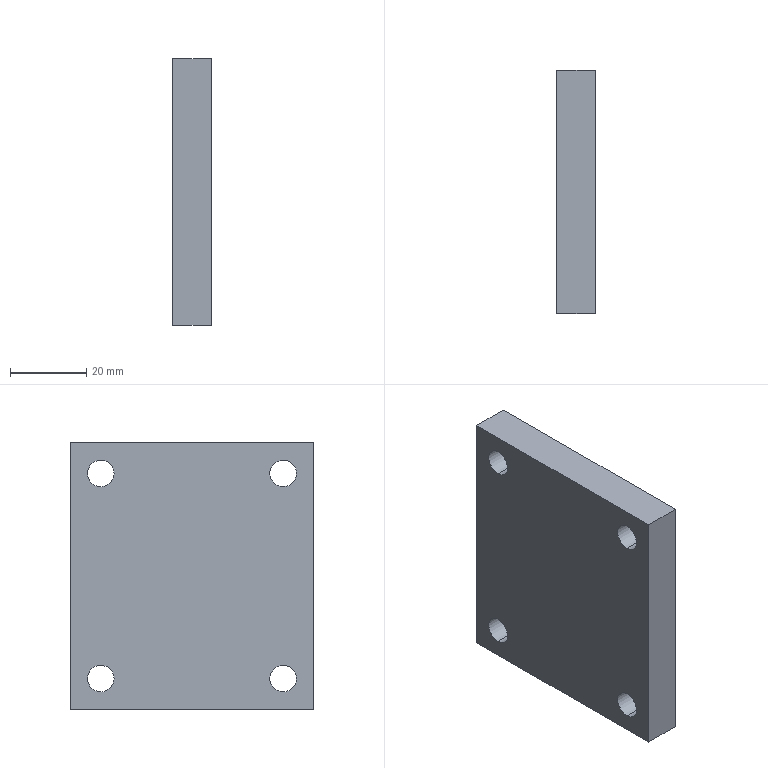Part | STEP file | Positioning_id2318_x_t | 1 solid | 14 faces | box 10 x 64 x 70 mm | volume 43261 mm3 | cylinder 8 | plane 6 | commonest cylinder face diameters 7 x8
STEP:
#1=CARTESIAN_POINT('',(0.,0.,0.));
#2=DIRECTION('',(0.,0.,1.));
#3=DIRECTION('',(1.,0.,0.));
#4=AXIS2_PLACEMENT_3D('',#1,#2,#3);
#5=CARTESIAN_POINT('',(-1013.002,324.,163.032));
#6=VERTEX_POINT('',#5);
#7=CARTESIAN_POINT('',(-1013.002,324.,170.032));
#8=VERTEX_POINT('',#7);
#9=CARTESIAN_POINT('',(-1013.002,324.,166.532));
#10=DIRECTION('',(1.,0.,0.));
#11=DIRECTION('',(0.,1.,0.));
#12=AXIS2_PLACEMENT_3D('',#9,#10,#11);
#13=CIRCLE('',#12,3.5);
#14=CARTESIAN_POINT('',(-1003.002,324.,166.532));
#15=DIRECTION('',(1.,0.,0.));
#16=DIRECTION('',(0.,0.,-1.));
#17=AXIS2_PLACEMENT_3D('',#14,#15,#16);
#18=CYLINDRICAL_SURFACE('',#17,3.5);
#19=CARTESIAN_POINT('',(-4.712,-10.));
#20=DIRECTION('',(1.,0.));
#21=VECTOR('',#20,1.);
#22=LINE('',#19,#21);
#23=(GEOMETRIC_REPRESENTATION_CONTEXT(2)PARAMETRIC_REPRESENTATION_CONTEXT()REPRESENTATION_CONTEXT('',''));
#24=DEFINITIONAL_REPRESENTATION('',(#22),#23);
#25=PCURVE('',#18,#24);
#26=CARTESIAN_POINT('',(-1013.002,284.,218.532));
#27=DIRECTION('',(-1.,0.,0.));
#28=DIRECTION('',(0.,-1.,0.));
#29=AXIS2_PLACEMENT_3D('',#26,#27,#28);
#30=PLANE('',#29);
#31=CARTESIAN_POINT('',(-43.5,-52.));
#32=CARTESIAN_POINT('',(-43.5,-45.938));
#33=CARTESIAN_POINT('',(-38.25,-48.969));
#34=CARTESIAN_POINT('',(-33.,-52.));
#35=CARTESIAN_POINT('',(-38.25,-55.031));
#36=CARTESIAN_POINT('',(-43.5,-58.062));
#37=CARTESIAN_POINT('',(-43.5,-52.));
#38=(BOUNDED_CURVE()B_SPLINE_CURVE(2,(#31,#32,#33,#34,#35,#36,#37),.UNSPECIFIED.,.T.,.F.)B_SPLINE_CURVE_WITH_KNOTS((1,2,2,2,2,1),(-2.094,0.,2.094,4.189,6.283,8.378),.UNSPECIFIED.)CURVE()GEOMETRIC_REPRESENTATION_ITEM()RATIONAL_B_SPLINE_CURVE((1.,0.5,1.,0.5,1.,0.5,1.))REPRESENTATION_ITEM(''));
#39=(GEOMETRIC_REPRESENTATION_CONTEXT(2)PARAMETRIC_REPRESENTATION_CONTEXT()REPRESENTATION_CONTEXT('',''));
#40=DEFINITIONAL_REPRESENTATION('',(#38),#39);
#41=PCURVE('',#30,#40);
#42=SURFACE_CURVE('',#13,(#25,#41),.PCURVE_S1.);
#43=EDGE_CURVE('',#6,#8,#42,.T.);
#44=ORIENTED_EDGE('',*,*,#43,.T.);
#45=CARTESIAN_POINT('',(-1003.002,324.,170.032));
#46=VERTEX_POINT('',#45);
#47=CARTESIAN_POINT('',(-1003.002,324.,170.032));
#48=DIRECTION('',(-1.,0.,0.));
#49=VECTOR('',#48,1.);
#50=LINE('',#47,#49);
#51=CARTESIAN_POINT('',(3.142,0.));
#52=DIRECTION('',(0.,-1.));
#53=VECTOR('',#52,1.);
#54=LINE('',#51,#53);
#55=(GEOMETRIC_REPRESENTATION_CONTEXT(2)PARAMETRIC_REPRESENTATION_CONTEXT()REPRESENTATION_CONTEXT('',''));
#56=DEFINITIONAL_REPRESENTATION('',(#54),#55);
#57=PCURVE('',#18,#56);
#58=CARTESIAN_POINT('',(-1003.002,324.,166.532));
#59=DIRECTION('',(1.,0.,0.));
#60=DIRECTION('',(0.,0.,-1.));
#61=AXIS2_PLACEMENT_3D('',#58,#59,#60);
#62=CYLINDRICAL_SURFACE('',#61,3.5);
#63=CARTESIAN_POINT('',(3.142,0.));
#64=DIRECTION('',(0.,-1.));
#65=VECTOR('',#64,1.);
#66=LINE('',#63,#65);
#67=(GEOMETRIC_REPRESENTATION_CONTEXT(2)PARAMETRIC_REPRESENTATION_CONTEXT()REPRESENTATION_CONTEXT('',''));
#68=DEFINITIONAL_REPRESENTATION('',(#66),#67);
#69=PCURVE('',#62,#68);
#70=SURFACE_CURVE('',#50,(#57,#69),.PCURVE_S1.);
#71=EDGE_CURVE('',#46,#8,#70,.T.);
#72=ORIENTED_EDGE('',*,*,#71,.F.);
#73=CARTESIAN_POINT('',(-1003.002,324.,163.032));
#74=VERTEX_POINT('',#73);
#75=CARTESIAN_POINT('',(-1003.002,324.,166.532));
#76=DIRECTION('',(1.,0.,0.));
#77=DIRECTION('',(0.,1.,0.));
#78=AXIS2_PLACEMENT_3D('',#75,#76,#77);
#79=CIRCLE('',#78,3.5);
#80=CARTESIAN_POINT('',(-4.712,0.));
#81=DIRECTION('',(1.,0.));
#82=VECTOR('',#81,1.);
#83=LINE('',#80,#82);
#84=(GEOMETRIC_REPRESENTATION_CONTEXT(2)PARAMETRIC_REPRESENTATION_CONTEXT()REPRESENTATION_CONTEXT('',''));
#85=DEFINITIONAL_REPRESENTATION('',(#83),#84);
#86=PCURVE('',#18,#85);
#87=CARTESIAN_POINT('',(-1003.002,284.,218.532));
#88=DIRECTION('',(1.,0.,0.));
#89=DIRECTION('',(0.,1.,0.));
#90=AXIS2_PLACEMENT_3D('',#87,#88,#89);
#91=PLANE('',#90);
#92=CARTESIAN_POINT('',(40.,-52.));
#93=DIRECTION('',(1.,0.));
#94=AXIS2_PLACEMENT_2D('',#92,#93);
#95=CIRCLE('',#94,3.5);
#96=(GEOMETRIC_REPRESENTATION_CONTEXT(2)PARAMETRIC_REPRESENTATION_CONTEXT()REPRESENTATION_CONTEXT('',''));
#97=DEFINITIONAL_REPRESENTATION('',(#95),#96);
#98=PCURVE('',#91,#97);
#99=SURFACE_CURVE('',#79,(#86,#98),.PCURVE_S1.);
#100=EDGE_CURVE('',#74,#46,#99,.T.);
#101=ORIENTED_EDGE('',*,*,#100,.F.);
#102=CARTESIAN_POINT('',(-1003.002,324.,163.032));
#103=DIRECTION('',(1.,0.,0.));
#104=VECTOR('',#103,1.);
#105=LINE('',#102,#104);
#106=CARTESIAN_POINT('',(0.,0.));
#107=DIRECTION('',(0.,1.));
#108=VECTOR('',#107,1.);
#109=LINE('',#106,#108);
#110=(GEOMETRIC_REPRESENTATION_CONTEXT(2)PARAMETRIC_REPRESENTATION_CONTEXT()REPRESENTATION_CONTEXT('',''));
#111=DEFINITIONAL_REPRESENTATION('',(#109),#110);
#112=PCURVE('',#18,#111);
#113=CARTESIAN_POINT('',(6.283,0.));
#114=DIRECTION('',(0.,1.));
#115=VECTOR('',#114,1.);
#116=LINE('',#113,#115);
#117=(GEOMETRIC_REPRESENTATION_CONTEXT(2)PARAMETRIC_REPRESENTATION_CONTEXT()REPRESENTATION_CONTEXT('',''));
#118=DEFINITIONAL_REPRESENTATION('',(#116),#117);
#119=PCURVE('',#62,#118);
#120=SURFACE_CURVE('',#105,(#112,#119),.PCURVE_S1.);
#121=EDGE_CURVE('',#6,#74,#120,.T.);
#122=ORIENTED_EDGE('',*,*,#121,.F.);
#123=EDGE_LOOP('',(#44,#72,#101,#122));
#124=FACE_BOUND('',#123,.F.);
#125=ADVANCED_FACE('',(#124),#18,.F.);
#126=CARTESIAN_POINT('',(-1013.002,324.,217.032));
#127=VERTEX_POINT('',#126);
#128=CARTESIAN_POINT('',(-1013.002,324.,224.032));
#129=VERTEX_POINT('',#128);
#130=CARTESIAN_POINT('',(-1013.002,324.,220.532));
#131=DIRECTION('',(1.,0.,0.));
#132=DIRECTION('',(0.,1.,0.));
#133=AXIS2_PLACEMENT_3D('',#130,#131,#132);
#134=CIRCLE('',#133,3.5);
#135=CARTESIAN_POINT('',(-1003.002,324.,220.532));
#136=DIRECTION('',(1.,0.,0.));
#137=DIRECTION('',(0.,0.,-1.));
#138=AXIS2_PLACEMENT_3D('',#135,#136,#137);
#139=CYLINDRICAL_SURFACE('',#138,3.5);
#140=CARTESIAN_POINT('',(-4.712,-10.));
#141=DIRECTION('',(1.,0.));
#142=VECTOR('',#141,1.);
#143=LINE('',#140,#142);
#144=(GEOMETRIC_REPRESENTATION_CONTEXT(2)PARAMETRIC_REPRESENTATION_CONTEXT()REPRESENTATION_CONTEXT('',''));
#145=DEFINITIONAL_REPRESENTATION('',(#143),#144);
#146=PCURVE('',#139,#145);
#147=CARTESIAN_POINT('',(-43.5,2.));
#148=CARTESIAN_POINT('',(-43.5,8.062));
#149=CARTESIAN_POINT('',(-38.25,5.031));
#150=CARTESIAN_POINT('',(-33.,2.));
#151=CARTESIAN_POINT('',(-38.25,-1.031));
#152=CARTESIAN_POINT('',(-43.5,-4.062));
#153=CARTESIAN_POINT('',(-43.5,2.));
#154=(BOUNDED_CURVE()B_SPLINE_CURVE(2,(#147,#148,#149,#150,#151,#152,#153),.UNSPECIFIED.,.T.,.F.)B_SPLINE_CURVE_WITH_KNOTS((1,2,2,2,2,1),(-2.094,0.,2.094,4.189,6.283,8.378),.UNSPECIFIED.)CURVE()GEOMETRIC_REPRESENTATION_ITEM()RATIONAL_B_SPLINE_CURVE((1.,0.5,1.,0.5,1.,0.5,1.))REPRESENTATION_ITEM(''));
#155=(GEOMETRIC_REPRESENTATION_CONTEXT(2)PARAMETRIC_REPRESENTATION_CONTEXT()REPRESENTATION_CONTEXT('',''));
#156=DEFINITIONAL_REPRESENTATION('',(#154),#155);
#157=PCURVE('',#30,#156);
#158=SURFACE_CURVE('',#134,(#146,#157),.PCURVE_S1.);
#159=EDGE_CURVE('',#127,#129,#158,.T.);
#160=ORIENTED_EDGE('',*,*,#159,.T.);
#161=CARTESIAN_POINT('',(-1003.002,324.,224.032));
#162=VERTEX_POINT('',#161);
#163=CARTESIAN_POINT('',(-1003.002,324.,224.032));
#164=DIRECTION('',(1.,0.,0.));
#165=VECTOR('',#164,1.);
#166=LINE('',#163,#165);
#167=CARTESIAN_POINT('',(3.142,0.));
#168=DIRECTION('',(0.,1.));
#169=VECTOR('',#168,1.);
#170=LINE('',#167,#169);
#171=(GEOMETRIC_REPRESENTATION_CONTEXT(2)PARAMETRIC_REPRESENTATION_CONTEXT()REPRESENTATION_CONTEXT('',''));
#172=DEFINITIONAL_REPRESENTATION('',(#170),#171);
#173=PCURVE('',#139,#172);
#174=CARTESIAN_POINT('',(-1003.002,324.,220.532));
#175=DIRECTION('',(1.,0.,0.));
#176=DIRECTION('',(0.,0.,-1.));
#177=AXIS2_PLACEMENT_3D('',#174,#175,#176);
#178=CYLINDRICAL_SURFACE('',#177,3.5);
#179=CARTESIAN_POINT('',(3.142,0.));
#180=DIRECTION('',(0.,1.));
#181=VECTOR('',#180,1.);
#182=LINE('',#179,#181);
#183=(GEOMETRIC_REPRESENTATION_CONTEXT(2)PARAMETRIC_REPRESENTATION_CONTEXT()REPRESENTATION_CONTEXT('',''));
#184=DEFINITIONAL_REPRESENTATION('',(#182),#183);
#185=PCURVE('',#178,#184);
#186=SURFACE_CURVE('',#166,(#173,#185),.PCURVE_S1.);
#187=EDGE_CURVE('',#129,#162,#186,.T.);
#188=ORIENTED_EDGE('',*,*,#187,.T.);
#189=CARTESIAN_POINT('',(-1003.002,324.,217.032));
#190=VERTEX_POINT('',#189);
#191=CARTESIAN_POINT('',(-1003.002,324.,220.532));
#192=DIRECTION('',(1.,0.,0.));
#193=DIRECTION('',(0.,1.,0.));
#194=AXIS2_PLACEMENT_3D('',#191,#192,#193);
#195=CIRCLE('',#194,3.5);
#196=CARTESIAN_POINT('',(-4.712,0.));
#197=DIRECTION('',(1.,0.));
#198=VECTOR('',#197,1.);
#199=LINE('',#196,#198);
#200=(GEOMETRIC_REPRESENTATION_CONTEXT(2)PARAMETRIC_REPRESENTATION_CONTEXT()REPRESENTATION_CONTEXT('',''));
#201=DEFINITIONAL_REPRESENTATION('',(#199),#200);
#202=PCURVE('',#139,#201);
#203=CARTESIAN_POINT('',(40.,2.));
#204=DIRECTION('',(1.,0.));
#205=AXIS2_PLACEMENT_2D('',#203,#204);
#206=CIRCLE('',#205,3.5);
#207=(GEOMETRIC_REPRESENTATION_CONTEXT(2)PARAMETRIC_REPRESENTATION_CONTEXT()REPRESENTATION_CONTEXT('',''));
#208=DEFINITIONAL_REPRESENTATION('',(#206),#207);
#209=PCURVE('',#91,#208);
#210=SURFACE_CURVE('',#195,(#202,#209),.PCURVE_S1.);
#211=EDGE_CURVE('',#190,#162,#210,.T.);
#212=ORIENTED_EDGE('',*,*,#211,.F.);
#213=CARTESIAN_POINT('',(-1003.002,324.,217.032));
#214=DIRECTION('',(-1.,0.,0.));
#215=VECTOR('',#214,1.);
#216=LINE('',#213,#215);
#217=CARTESIAN_POINT('',(0.,0.));
#218=DIRECTION('',(0.,-1.));
#219=VECTOR('',#218,1.);
#220=LINE('',#217,#219);
#221=(GEOMETRIC_REPRESENTATION_CONTEXT(2)PARAMETRIC_REPRESENTATION_CONTEXT()REPRESENTATION_CONTEXT('',''));
#222=DEFINITIONAL_REPRESENTATION('',(#220),#221);
#223=PCURVE('',#139,#222);
#224=CARTESIAN_POINT('',(6.283,0.));
#225=DIRECTION('',(0.,-1.));
#226=VECTOR('',#225,1.);
#227=LINE('',#224,#226);
#228=(GEOMETRIC_REPRESENTATION_CONTEXT(2)PARAMETRIC_REPRESENTATION_CONTEXT()REPRESENTATION_CONTEXT('',''));
#229=DEFINITIONAL_REPRESENTATION('',(#227),#228);
#230=PCURVE('',#178,#229);
#231=SURFACE_CURVE('',#216,(#223,#230),.PCURVE_S1.);
#232=EDGE_CURVE('',#190,#127,#231,.T.);
#233=ORIENTED_EDGE('',*,*,#232,.T.);
#234=EDGE_LOOP('',(#160,#188,#212,#233));
#235=FACE_BOUND('',#234,.F.);
#236=ADVANCED_FACE('',(#235),#139,.F.);
#237=CARTESIAN_POINT('',(-1013.002,276.,217.032));
#238=VERTEX_POINT('',#237);
#239=CARTESIAN_POINT('',(-1013.002,276.,224.032));
#240=VERTEX_POINT('',#239);
#241=CARTESIAN_POINT('',(-1013.002,276.,220.532));
#242=DIRECTION('',(1.,0.,0.));
#243=DIRECTION('',(0.,1.,0.));
#244=AXIS2_PLACEMENT_3D('',#241,#242,#243);
#245=CIRCLE('',#244,3.5);
#246=CARTESIAN_POINT('',(-1003.002,276.,220.532));
#247=DIRECTION('',(1.,0.,0.));
#248=DIRECTION('',(0.,0.,-1.));
#249=AXIS2_PLACEMENT_3D('',#246,#247,#248);
#250=CYLINDRICAL_SURFACE('',#249,3.5);
#251=CARTESIAN_POINT('',(-4.712,-10.));
#252=DIRECTION('',(1.,0.));
#253=VECTOR('',#252,1.);
#254=LINE('',#251,#253);
#255=(GEOMETRIC_REPRESENTATION_CONTEXT(2)PARAMETRIC_REPRESENTATION_CONTEXT()REPRESENTATION_CONTEXT('',''));
#256=DEFINITIONAL_REPRESENTATION('',(#254),#255);
#257=PCURVE('',#250,#256);
#258=CARTESIAN_POINT('',(4.5,2.));
#259=CARTESIAN_POINT('',(4.5,8.062));
#260=CARTESIAN_POINT('',(9.75,5.031));
#261=CARTESIAN_POINT('',(15.,2.));
#262=CARTESIAN_POINT('',(9.75,-1.031));
#263=CARTESIAN_POINT('',(4.5,-4.062));
#264=CARTESIAN_POINT('',(4.5,2.));
#265=(BOUNDED_CURVE()B_SPLINE_CURVE(2,(#258,#259,#260,#261,#262,#263,#264),.UNSPECIFIED.,.T.,.F.)B_SPLINE_CURVE_WITH_KNOTS((1,2,2,2,2,1),(-2.094,0.,2.094,4.189,6.283,8.378),.UNSPECIFIED.)CURVE()GEOMETRIC_REPRESENTATION_ITEM()RATIONAL_B_SPLINE_CURVE((1.,0.5,1.,0.5,1.,0.5,1.))REPRESENTATION_ITEM(''));
#266=(GEOMETRIC_REPRESENTATION_CONTEXT(2)PARAMETRIC_REPRESENTATION_CONTEXT()REPRESENTATION_CONTEXT('',''));
#267=DEFINITIONAL_REPRESENTATION('',(#265),#266);
#268=PCURVE('',#30,#267);
#269=SURFACE_CURVE('',#245,(#257,#268),.PCURVE_S1.);
#270=EDGE_CURVE('',#238,#240,#269,.T.);
#271=ORIENTED_EDGE('',*,*,#270,.T.);
#272=CARTESIAN_POINT('',(-1003.002,276.,224.032));
#273=VERTEX_POINT('',#272);
#274=CARTESIAN_POINT('',(-1003.002,276.,224.032));
#275=DIRECTION('',(-1.,0.,0.));
#276=VECTOR('',#275,1.);
#277=LINE('',#274,#276);
#278=CARTESIAN_POINT('',(3.142,0.));
#279=DIRECTION('',(0.,-1.));
#280=VECTOR('',#279,1.);
#281=LINE('',#278,#280);
#282=(GEOMETRIC_REPRESENTATION_CONTEXT(2)PARAMETRIC_REPRESENTATION_CONTEXT()REPRESENTATION_CONTEXT('',''));
#283=DEFINITIONAL_REPRESENTATION('',(#281),#282);
#284=PCURVE('',#250,#283);
#285=CARTESIAN_POINT('',(-1003.002,276.,220.532));
#286=DIRECTION('',(1.,0.,0.));
#287=DIRECTION('',(0.,0.,-1.));
#288=AXIS2_PLACEMENT_3D('',#285,#286,#287);
#289=CYLINDRICAL_SURFACE('',#288,3.5);
#290=CARTESIAN_POINT('',(3.142,0.));
#291=DIRECTION('',(0.,-1.));
#292=VECTOR('',#291,1.);
#293=LINE('',#290,#292);
#294=(GEOMETRIC_REPRESENTATION_CONTEXT(2)PARAMETRIC_REPRESENTATION_CONTEXT()REPRESENTATION_CONTEXT('',''));
#295=DEFINITIONAL_REPRESENTATION('',(#293),#294);
#296=PCURVE('',#289,#295);
#297=SURFACE_CURVE('',#277,(#284,#296),.PCURVE_S1.);
#298=EDGE_CURVE('',#273,#240,#297,.T.);
#299=ORIENTED_EDGE('',*,*,#298,.F.);
#300=CARTESIAN_POINT('',(-1003.002,276.,217.032));
#301=VERTEX_POINT('',#300);
#302=CARTESIAN_POINT('',(-1003.002,276.,220.532));
#303=DIRECTION('',(1.,0.,0.));
#304=DIRECTION('',(0.,1.,0.));
#305=AXIS2_PLACEMENT_3D('',#302,#303,#304);
#306=CIRCLE('',#305,3.5);
#307=CARTESIAN_POINT('',(-4.712,0.));
#308=DIRECTION('',(1.,0.));
#309=VECTOR('',#308,1.);
#310=LINE('',#307,#309);
#311=(GEOMETRIC_REPRESENTATION_CONTEXT(2)PARAMETRIC_REPRESENTATION_CONTEXT()REPRESENTATION_CONTEXT('',''));
#312=DEFINITIONAL_REPRESENTATION('',(#310),#311);
#313=PCURVE('',#250,#312);
#314=CARTESIAN_POINT('',(-8.,2.));
#315=DIRECTION('',(1.,0.));
#316=AXIS2_PLACEMENT_2D('',#314,#315);
#317=CIRCLE('',#316,3.5);
#318=(GEOMETRIC_REPRESENTATION_CONTEXT(2)PARAMETRIC_REPRESENTATION_CONTEXT()REPRESENTATION_CONTEXT('',''));
#319=DEFINITIONAL_REPRESENTATION('',(#317),#318);
#320=PCURVE('',#91,#319);
#321=SURFACE_CURVE('',#306,(#313,#320),.PCURVE_S1.);
#322=EDGE_CURVE('',#301,#273,#321,.T.);
#323=ORIENTED_EDGE('',*,*,#322,.F.);
#324=CARTESIAN_POINT('',(-1003.002,276.,217.032));
#325=DIRECTION('',(1.,0.,0.));
#326=VECTOR('',#325,1.);
#327=LINE('',#324,#326);
#328=CARTESIAN_POINT('',(0.,0.));
#329=DIRECTION('',(0.,1.));
#330=VECTOR('',#329,1.);
#331=LINE('',#328,#330);
#332=(GEOMETRIC_REPRESENTATION_CONTEXT(2)PARAMETRIC_REPRESENTATION_CONTEXT()REPRESENTATION_CONTEXT('',''));
#333=DEFINITIONAL_REPRESENTATION('',(#331),#332);
#334=PCURVE('',#250,#333);
#335=CARTESIAN_POINT('',(6.283,0.));
#336=DIRECTION('',(0.,1.));
#337=VECTOR('',#336,1.);
#338=LINE('',#335,#337);
#339=(GEOMETRIC_REPRESENTATION_CONTEXT(2)PARAMETRIC_REPRESENTATION_CONTEXT()REPRESENTATION_CONTEXT('',''));
#340=DEFINITIONAL_REPRESENTATION('',(#338),#339);
#341=PCURVE('',#289,#340);
#342=SURFACE_CURVE('',#327,(#334,#341),.PCURVE_S1.);
#343=EDGE_CURVE('',#238,#301,#342,.T.);
#344=ORIENTED_EDGE('',*,*,#343,.F.);
#345=EDGE_LOOP('',(#271,#299,#323,#344));
#346=FACE_BOUND('',#345,.F.);
#347=ADVANCED_FACE('',(#346),#250,.F.);
#348=CARTESIAN_POINT('',(-1013.002,276.,163.032));
#349=VERTEX_POINT('',#348);
#350=CARTESIAN_POINT('',(-1013.002,276.,170.032));
#351=VERTEX_POINT('',#350);
#352=CARTESIAN_POINT('',(-1013.002,276.,166.532));
#353=DIRECTION('',(1.,0.,0.));
#354=DIRECTION('',(0.,1.,0.));
#355=AXIS2_PLACEMENT_3D('',#352,#353,#354);
#356=CIRCLE('',#355,3.5);
#357=CARTESIAN_POINT('',(-1003.002,276.,166.532));
#358=DIRECTION('',(1.,0.,0.));
#359=DIRECTION('',(0.,0.,-1.));
#360=AXIS2_PLACEMENT_3D('',#357,#358,#359);
#361=CYLINDRICAL_SURFACE('',#360,3.5);
#362=CARTESIAN_POINT('',(-4.712,-10.));
#363=DIRECTION('',(1.,0.));
#364=VECTOR('',#363,1.);
#365=LINE('',#362,#364);
#366=(GEOMETRIC_REPRESENTATION_CONTEXT(2)PARAMETRIC_REPRESENTATION_CONTEXT()REPRESENTATION_CONTEXT('',''));
#367=DEFINITIONAL_REPRESENTATION('',(#365),#366);
#368=PCURVE('',#361,#367);
#369=CARTESIAN_POINT('',(4.5,-52.));
#370=CARTESIAN_POINT('',(4.5,-45.938));
#371=CARTESIAN_POINT('',(9.75,-48.969));
#372=CARTESIAN_POINT('',(15.,-52.));
#373=CARTESIAN_POINT('',(9.75,-55.031));
#374=CARTESIAN_POINT('',(4.5,-58.062));
#375=CARTESIAN_POINT('',(4.5,-52.));
#376=(BOUNDED_CURVE()B_SPLINE_CURVE(2,(#369,#370,#371,#372,#373,#374,#375),.UNSPECIFIED.,.T.,.F.)B_SPLINE_CURVE_WITH_KNOTS((1,2,2,2,2,1),(-2.094,0.,2.094,4.189,6.283,8.378),.UNSPECIFIED.)CURVE()GEOMETRIC_REPRESENTATION_ITEM()RATIONAL_B_SPLINE_CURVE((1.,0.5,1.,0.5,1.,0.5,1.))REPRESENTATION_ITEM(''));
#377=(GEOMETRIC_REPRESENTATION_CONTEXT(2)PARAMETRIC_REPRESENTATION_CONTEXT()REPRESENTATION_CONTEXT('',''));
#378=DEFINITIONAL_REPRESENTATION('',(#376),#377);
#379=PCURVE('',#30,#378);
#380=SURFACE_CURVE('',#356,(#368,#379),.PCURVE_S1.);
#381=EDGE_CURVE('',#349,#351,#380,.T.);
#382=ORIENTED_EDGE('',*,*,#381,.T.);
#383=CARTESIAN_POINT('',(-1003.002,276.,170.032));
#384=VERTEX_POINT('',#383);
#385=CARTESIAN_POINT('',(-1003.002,276.,170.032));
#386=DIRECTION('',(-1.,0.,0.));
#387=VECTOR('',#386,1.);
#388=LINE('',#385,#387);
#389=CARTESIAN_POINT('',(3.142,0.));
#390=DIRECTION('',(0.,-1.));
#391=VECTOR('',#390,1.);
#392=LINE('',#389,#391);
#393=(GEOMETRIC_REPRESENTATION_CONTEXT(2)PARAMETRIC_REPRESENTATION_CONTEXT()REPRESENTATION_CONTEXT('',''));
#394=DEFINITIONAL_REPRESENTATION('',(#392),#393);
#395=PCURVE('',#361,#394);
#396=CARTESIAN_POINT('',(-1003.002,276.,166.532));
#397=DIRECTION('',(1.,0.,0.));
#398=DIRECTION('',(0.,0.,-1.));
#399=AXIS2_PLACEMENT_3D('',#396,#397,#398);
#400=CYLINDRICAL_SURFACE('',#399,3.5);
#401=CARTESIAN_POINT('',(3.142,0.));
#402=DIRECTION('',(0.,-1.));
#403=VECTOR('',#402,1.);
#404=LINE('',#401,#403);
#405=(GEOMETRIC_REPRESENTATION_CONTEXT(2)PARAMETRIC_REPRESENTATION_CONTEXT()REPRESENTATION_CONTEXT('',''));
#406=DEFINITIONAL_REPRESENTATION('',(#404),#405);
#407=PCURVE('',#400,#406);
#408=SURFACE_CURVE('',#388,(#395,#407),.PCURVE_S1.);
#409=EDGE_CURVE('',#384,#351,#408,.T.);
#410=ORIENTED_EDGE('',*,*,#409,.F.);
#411=CARTESIAN_POINT('',(-1003.002,276.,163.032));
#412=VERTEX_POINT('',#411);
#413=CARTESIAN_POINT('',(-1003.002,276.,166.532));
#414=DIRECTION('',(1.,0.,0.));
#415=DIRECTION('',(0.,1.,0.));
#416=AXIS2_PLACEMENT_3D('',#413,#414,#415);
#417=CIRCLE('',#416,3.5);
#418=CARTESIAN_POINT('',(-4.712,0.));
#419=DIRECTION('',(1.,0.));
#420=VECTOR('',#419,1.);
#421=LINE('',#418,#420);
#422=(GEOMETRIC_REPRESENTATION_CONTEXT(2)PARAMETRIC_REPRESENTATION_CONTEXT()REPRESENTATION_CONTEXT('',''));
#423=DEFINITIONAL_REPRESENTATION('',(#421),#422);
#424=PCURVE('',#361,#423);
#425=CARTESIAN_POINT('',(-8.,-52.));
#426=DIRECTION('',(1.,0.));
#427=AXIS2_PLACEMENT_2D('',#425,#426);
#428=CIRCLE('',#427,3.5);
#429=(GEOMETRIC_REPRESENTATION_CONTEXT(2)PARAMETRIC_REPRESENTATION_CONTEXT()REPRESENTATION_CONTEXT('',''));
#430=DEFINITIONAL_REPRESENTATION('',(#428),#429);
#431=PCURVE('',#91,#430);
#432=SURFACE_CURVE('',#417,(#424,#431),.PCURVE_S1.);
#433=EDGE_CURVE('',#412,#384,#432,.T.);
#434=ORIENTED_EDGE('',*,*,#433,.F.);
#435=CARTESIAN_POINT('',(-1003.002,276.,163.032));
#436=DIRECTION('',(1.,0.,0.));
#437=VECTOR('',#436,1.);
#438=LINE('',#435,#437);
#439=CARTESIAN_POINT('',(0.,0.));
#440=DIRECTION('',(0.,1.));
#441=VECTOR('',#440,1.);
#442=LINE('',#439,#441);
#443=(GEOMETRIC_REPRESENTATION_CONTEXT(2)PARAMETRIC_REPRESENTATION_CONTEXT()REPRESENTATION_CONTEXT('',''));
#444=DEFINITIONAL_REPRESENTATION('',(#442),#443);
#445=PCURVE('',#361,#444);
#446=CARTESIAN_POINT('',(6.283,0.));
#447=DIRECTION('',(0.,1.));
#448=VECTOR('',#447,1.);
#449=LINE('',#446,#448);
#450=(GEOMETRIC_REPRESENTATION_CONTEXT(2)PARAMETRIC_REPRESENTATION_CONTEXT()REPRESENTATION_CONTEXT('',''));
#451=DEFINITIONAL_REPRESENTATION('',(#449),#450);
#452=PCURVE('',#400,#451);
#453=SURFACE_CURVE('',#438,(#445,#452),.PCURVE_S1.);
#454=EDGE_CURVE('',#349,#412,#453,.T.);
#455=ORIENTED_EDGE('',*,*,#454,.F.);
#456=EDGE_LOOP('',(#382,#410,#434,#455));
#457=FACE_BOUND('',#456,.F.);
#458=ADVANCED_FACE('',(#457),#361,.F.);
#459=CARTESIAN_POINT('',(-1013.002,268.,158.532));
#460=VERTEX_POINT('',#459);
#461=CARTESIAN_POINT('',(-1013.002,268.,228.532));
#462=VERTEX_POINT('',#461);
#463=CARTESIAN_POINT('',(-1013.002,268.,158.532));
#464=DIRECTION('',(0.,0.,1.));
#465=VECTOR('',#464,1.);
#466=LINE('',#463,#465);
#467=CARTESIAN_POINT('',(-1013.002,268.,218.532));
#468=DIRECTION('',(0.,-1.,0.));
#469=DIRECTION('',(1.,0.,0.));
#470=AXIS2_PLACEMENT_3D('',#467,#468,#469);
#471=PLANE('',#470);
#472=CARTESIAN_POINT('',(0.,-60.));
#473=DIRECTION('',(0.,1.));
#474=VECTOR('',#473,1.);
#475=LINE('',#472,#474);
#476=(GEOMETRIC_REPRESENTATION_CONTEXT(2)PARAMETRIC_REPRESENTATION_CONTEXT()REPRESENTATION_CONTEXT('',''));
#477=DEFINITIONAL_REPRESENTATION('',(#475),#476);
#478=PCURVE('',#471,#477);
#479=CARTESIAN_POINT('',(16.,-60.));
#480=DIRECTION('',(0.,1.));
#481=VECTOR('',#480,1.);
#482=LINE('',#479,#481);
#483=(GEOMETRIC_REPRESENTATION_CONTEXT(2)PARAMETRIC_REPRESENTATION_CONTEXT()REPRESENTATION_CONTEXT('',''));
#484=DEFINITIONAL_REPRESENTATION('',(#482),#483);
#485=PCURVE('',#30,#484);
#486=SURFACE_CURVE('',#466,(#478,#485),.PCURVE_S1.);
#487=EDGE_CURVE('',#460,#462,#486,.T.);
#488=ORIENTED_EDGE('',*,*,#487,.F.);
#489=CARTESIAN_POINT('',(-1003.002,268.,158.532));
#490=VERTEX_POINT('',#489);
#491=CARTESIAN_POINT('',(-1013.002,268.,158.532));
#492=DIRECTION('',(1.,0.,0.));
#493=VECTOR('',#492,1.);
#494=LINE('',#491,#493);
#495=CARTESIAN_POINT('',(0.,-60.));
#496=DIRECTION('',(1.,0.));
#497=VECTOR('',#496,1.);
#498=LINE('',#495,#497);
#499=(GEOMETRIC_REPRESENTATION_CONTEXT(2)PARAMETRIC_REPRESENTATION_CONTEXT()REPRESENTATION_CONTEXT('',''));
#500=DEFINITIONAL_REPRESENTATION('',(#498),#499);
#501=PCURVE('',#471,#500);
#502=CARTESIAN_POINT('',(-1013.002,284.,158.532));
#503=DIRECTION('',(0.,0.,-1.));
#504=DIRECTION('',(1.,0.,0.));
#505=AXIS2_PLACEMENT_3D('',#502,#503,#504);
#506=PLANE('',#505);
#507=CARTESIAN_POINT('',(0.,16.));
#508=DIRECTION('',(1.,0.));
#509=VECTOR('',#508,1.);
#510=LINE('',#507,#509);
#511=(GEOMETRIC_REPRESENTATION_CONTEXT(2)PARAMETRIC_REPRESENTATION_CONTEXT()REPRESENTATION_CONTEXT('',''));
#512=DEFINITIONAL_REPRESENTATION('',(#510),#511);
#513=PCURVE('',#506,#512);
#514=SURFACE_CURVE('',#494,(#501,#513),.PCURVE_S1.);
#515=EDGE_CURVE('',#460,#490,#514,.T.);
#516=ORIENTED_EDGE('',*,*,#515,.T.);
#517=CARTESIAN_POINT('',(-1003.002,268.,228.532));
#518=VERTEX_POINT('',#517);
#519=CARTESIAN_POINT('',(-1003.002,268.,228.532));
#520=DIRECTION('',(0.,0.,-1.));
#521=VECTOR('',#520,1.);
#522=LINE('',#519,#521);
#523=CARTESIAN_POINT('',(10.,10.));
#524=DIRECTION('',(0.,-1.));
#525=VECTOR('',#524,1.);
#526=LINE('',#523,#525);
#527=(GEOMETRIC_REPRESENTATION_CONTEXT(2)PARAMETRIC_REPRESENTATION_CONTEXT()REPRESENTATION_CONTEXT('',''));
#528=DEFINITIONAL_REPRESENTATION('',(#526),#527);
#529=PCURVE('',#471,#528);
#530=CARTESIAN_POINT('',(-16.,10.));
#531=DIRECTION('',(0.,-1.));
#532=VECTOR('',#531,1.);
#533=LINE('',#530,#532);
#534=(GEOMETRIC_REPRESENTATION_CONTEXT(2)PARAMETRIC_REPRESENTATION_CONTEXT()REPRESENTATION_CONTEXT('',''));
#535=DEFINITIONAL_REPRESENTATION('',(#533),#534);
#536=PCURVE('',#91,#535);
#537=SURFACE_CURVE('',#522,(#529,#536),.PCURVE_S1.);
#538=EDGE_CURVE('',#518,#490,#537,.T.);
#539=ORIENTED_EDGE('',*,*,#538,.F.);
#540=CARTESIAN_POINT('',(-1013.002,268.,228.532));
#541=DIRECTION('',(1.,0.,0.));
#542=VECTOR('',#541,1.);
#543=LINE('',#540,#542);
#544=CARTESIAN_POINT('',(0.,10.));
#545=DIRECTION('',(1.,0.));
#546=VECTOR('',#545,1.);
#547=LINE('',#544,#546);
#548=(GEOMETRIC_REPRESENTATION_CONTEXT(2)PARAMETRIC_REPRESENTATION_CONTEXT()REPRESENTATION_CONTEXT('',''));
#549=DEFINITIONAL_REPRESENTATION('',(#547),#548);
#550=PCURVE('',#471,#549);
#551=CARTESIAN_POINT('',(-1013.002,284.,228.532));
#552=DIRECTION('',(0.,0.,1.));
#553=DIRECTION('',(-1.,0.,0.));
#554=AXIS2_PLACEMENT_3D('',#551,#552,#553);
#555=PLANE('',#554);
#556=CARTESIAN_POINT('',(0.,16.));
#557=DIRECTION('',(-1.,0.));
#558=VECTOR('',#557,1.);
#559=LINE('',#556,#558);
#560=(GEOMETRIC_REPRESENTATION_CONTEXT(2)PARAMETRIC_REPRESENTATION_CONTEXT()REPRESENTATION_CONTEXT('',''));
#561=DEFINITIONAL_REPRESENTATION('',(#559),#560);
#562=PCURVE('',#555,#561);
#563=SURFACE_CURVE('',#543,(#550,#562),.PCURVE_S1.);
#564=EDGE_CURVE('',#462,#518,#563,.T.);
#565=ORIENTED_EDGE('',*,*,#564,.F.);
#566=EDGE_LOOP('',(#488,#516,#539,#565));
#567=FACE_BOUND('',#566,.T.);
#568=ADVANCED_FACE('',(#567),#471,.T.);
#569=CARTESIAN_POINT('',(-1013.002,276.,170.032));
#570=CARTESIAN_POINT('',(-1013.002,272.5,170.032));
#571=CARTESIAN_POINT('',(-1013.002,270.75,166.532));
#572=CARTESIAN_POINT('',(-1013.002,272.5,163.032));
#573=CARTESIAN_POINT('',(-1013.002,276.,163.032));
#574=(BOUNDED_CURVE()B_SPLINE_CURVE(4,(#569,#570,#571,#572,#573),.UNSPECIFIED.,.F.,.F.)B_SPLINE_CURVE_WITH_KNOTS((5,5),(0.,1.),.PIECEWISE_BEZIER_KNOTS.)CURVE()GEOMETRIC_REPRESENTATION_ITEM()RATIONAL_B_SPLINE_CURVE((1.,0.7071,0.6667,0.7071,1.))REPRESENTATION_ITEM(''));
#575=CARTESIAN_POINT('',(8.,-48.5));
#576=CARTESIAN_POINT('',(11.5,-48.5));
#577=CARTESIAN_POINT('',(13.25,-52.));
#578=CARTESIAN_POINT('',(11.5,-55.5));
#579=CARTESIAN_POINT('',(8.,-55.5));
#580=(BOUNDED_CURVE()B_SPLINE_CURVE(4,(#575,#576,#577,#578,#579),.UNSPECIFIED.,.F.,.F.)B_SPLINE_CURVE_WITH_KNOTS((5,5),(0.,1.),.PIECEWISE_BEZIER_KNOTS.)CURVE()GEOMETRIC_REPRESENTATION_ITEM()RATIONAL_B_SPLINE_CURVE((1.,0.7071,0.6667,0.7071,1.))REPRESENTATION_ITEM(''));
#581=(GEOMETRIC_REPRESENTATION_CONTEXT(2)PARAMETRIC_REPRESENTATION_CONTEXT()REPRESENTATION_CONTEXT('',''));
#582=DEFINITIONAL_REPRESENTATION('',(#580),#581);
#583=PCURVE('',#30,#582);
#584=CARTESIAN_POINT('',(3.142,-10.));
#585=CARTESIAN_POINT('',(3.184,-10.));
#586=CARTESIAN_POINT('',(3.271,-10.));
#587=CARTESIAN_POINT('',(3.405,-10.));
#588=CARTESIAN_POINT('',(3.542,-10.));
#589=CARTESIAN_POINT('',(3.681,-10.));
#590=CARTESIAN_POINT('',(3.823,-10.));
#591=CARTESIAN_POINT('',(3.968,-10.));
#592=CARTESIAN_POINT('',(4.114,-10.));
#593=CARTESIAN_POINT('',(4.262,-10.));
#594=CARTESIAN_POINT('',(4.412,-10.));
#595=CARTESIAN_POINT('',(4.562,-10.));
#596=CARTESIAN_POINT('',(4.712,-10.));
#597=CARTESIAN_POINT('',(4.863,-10.));
#598=CARTESIAN_POINT('',(5.013,-10.));
#599=CARTESIAN_POINT('',(5.163,-10.));
#600=CARTESIAN_POINT('',(5.311,-10.));
#601=CARTESIAN_POINT('',(5.457,-10.));
#602=CARTESIAN_POINT('',(5.602,-10.));
#603=CARTESIAN_POINT('',(5.744,-10.));
#604=CARTESIAN_POINT('',(5.883,-10.));
#605=CARTESIAN_POINT('',(6.02,-10.));
#606=CARTESIAN_POINT('',(6.153,-10.));
#607=CARTESIAN_POINT('',(6.24,-10.));
#608=CARTESIAN_POINT('',(6.283,-10.));
#609=B_SPLINE_CURVE_WITH_KNOTS('',3,(#584,#585,#586,#587,#588,#589,#590,#591,#592,#593,#594,#595,#596,#597,#598,#599,#600,#601,#602,#603,#604,#605,#606,#607,#608),.UNSPECIFIED.,.F.,.F.,(4,1,1,1,1,1,1,1,1,1,1,1,1,1,1,1,1,1,1,1,1,1,4),(0.,0.04545,0.09091,0.1364,0.1818,0.2273,0.2727,0.3182,0.3636,0.4091,0.4545,0.5,0.5455,0.5909,0.6364,0.6818,0.7273,0.7727,0.8182,0.8636,0.9091,0.9545,1.),.QUASI_UNIFORM_KNOTS.);
#610=(GEOMETRIC_REPRESENTATION_CONTEXT(2)PARAMETRIC_REPRESENTATION_CONTEXT()REPRESENTATION_CONTEXT('',''));
#611=DEFINITIONAL_REPRESENTATION('',(#609),#610);
#612=PCURVE('',#400,#611);
#613=SURFACE_CURVE('',#574,(#583,#612),.PCURVE_S1.);
#614=EDGE_CURVE('',#351,#349,#613,.T.);
#615=ORIENTED_EDGE('',*,*,#614,.T.);
#616=ORIENTED_EDGE('',*,*,#381,.T.);
#617=EDGE_LOOP('',(#615,#616));
#618=FACE_BOUND('',#617,.T.);
#619=CARTESIAN_POINT('',(-1013.002,276.,224.032));
#620=CARTESIAN_POINT('',(-1013.002,272.5,224.032));
#621=CARTESIAN_POINT('',(-1013.002,270.75,220.532));
#622=CARTESIAN_POINT('',(-1013.002,272.5,217.032));
#623=CARTESIAN_POINT('',(-1013.002,276.,217.032));
#624=(BOUNDED_CURVE()B_SPLINE_CURVE(4,(#619,#620,#621,#622,#623),.UNSPECIFIED.,.F.,.F.)B_SPLINE_CURVE_WITH_KNOTS((5,5),(0.,1.),.PIECEWISE_BEZIER_KNOTS.)CURVE()GEOMETRIC_REPRESENTATION_ITEM()RATIONAL_B_SPLINE_CURVE((1.,0.7071,0.6667,0.7071,1.))REPRESENTATION_ITEM(''));
#625=CARTESIAN_POINT('',(8.,5.5));
#626=CARTESIAN_POINT('',(11.5,5.5));
#627=CARTESIAN_POINT('',(13.25,2.));
#628=CARTESIAN_POINT('',(11.5,-1.5));
#629=CARTESIAN_POINT('',(8.,-1.5));
#630=(BOUNDED_CURVE()B_SPLINE_CURVE(4,(#625,#626,#627,#628,#629),.UNSPECIFIED.,.F.,.F.)B_SPLINE_CURVE_WITH_KNOTS((5,5),(0.,1.),.PIECEWISE_BEZIER_KNOTS.)CURVE()GEOMETRIC_REPRESENTATION_ITEM()RATIONAL_B_SPLINE_CURVE((1.,0.7071,0.6667,0.7071,1.))REPRESENTATION_ITEM(''));
#631=(GEOMETRIC_REPRESENTATION_CONTEXT(2)PARAMETRIC_REPRESENTATION_CONTEXT()REPRESENTATION_CONTEXT('',''));
#632=DEFINITIONAL_REPRESENTATION('',(#630),#631);
#633=PCURVE('',#30,#632);
#634=CARTESIAN_POINT('',(3.142,-10.));
#635=CARTESIAN_POINT('',(3.184,-10.));
#636=CARTESIAN_POINT('',(3.271,-10.));
#637=CARTESIAN_POINT('',(3.405,-10.));
#638=CARTESIAN_POINT('',(3.542,-10.));
#639=CARTESIAN_POINT('',(3.681,-10.));
#640=CARTESIAN_POINT('',(3.823,-10.));
#641=CARTESIAN_POINT('',(3.968,-10.));
#642=CARTESIAN_POINT('',(4.114,-10.));
#643=CARTESIAN_POINT('',(4.262,-10.));
#644=CARTESIAN_POINT('',(4.412,-10.));
#645=CARTESIAN_POINT('',(4.562,-10.));
#646=CARTESIAN_POINT('',(4.712,-10.));
#647=CARTESIAN_POINT('',(4.863,-10.));
#648=CARTESIAN_POINT('',(5.013,-10.));
#649=CARTESIAN_POINT('',(5.163,-10.));
#650=CARTESIAN_POINT('',(5.311,-10.));
#651=CARTESIAN_POINT('',(5.457,-10.));
#652=CARTESIAN_POINT('',(5.602,-10.));
#653=CARTESIAN_POINT('',(5.744,-10.));
#654=CARTESIAN_POINT('',(5.883,-10.));
#655=CARTESIAN_POINT('',(6.02,-10.));
#656=CARTESIAN_POINT('',(6.153,-10.));
#657=CARTESIAN_POINT('',(6.24,-10.));
#658=CARTESIAN_POINT('',(6.283,-10.));
#659=B_SPLINE_CURVE_WITH_KNOTS('',3,(#634,#635,#636,#637,#638,#639,#640,#641,#642,#643,#644,#645,#646,#647,#648,#649,#650,#651,#652,#653,#654,#655,#656,#657,#658),.UNSPECIFIED.,.F.,.F.,(4,1,1,1,1,1,1,1,1,1,1,1,1,1,1,1,1,1,1,1,1,1,4),(0.,0.04545,0.09091,0.1364,0.1818,0.2273,0.2727,0.3182,0.3636,0.4091,0.4545,0.5,0.5455,0.5909,0.6364,0.6818,0.7273,0.7727,0.8182,0.8636,0.9091,0.9545,1.),.QUASI_UNIFORM_KNOTS.);
#660=(GEOMETRIC_REPRESENTATION_CONTEXT(2)PARAMETRIC_REPRESENTATION_CONTEXT()REPRESENTATION_CONTEXT('',''));
#661=DEFINITIONAL_REPRESENTATION('',(#659),#660);
#662=PCURVE('',#289,#661);
#663=SURFACE_CURVE('',#624,(#633,#662),.PCURVE_S1.);
#664=EDGE_CURVE('',#240,#238,#663,.T.);
#665=ORIENTED_EDGE('',*,*,#664,.T.);
#666=ORIENTED_EDGE('',*,*,#270,.T.);
#667=EDGE_LOOP('',(#665,#666));
#668=FACE_BOUND('',#667,.T.);
#669=CARTESIAN_POINT('',(-1013.002,324.,224.032));
#670=CARTESIAN_POINT('',(-1013.002,320.5,224.032));
#671=CARTESIAN_POINT('',(-1013.002,318.75,220.532));
#672=CARTESIAN_POINT('',(-1013.002,320.5,217.032));
#673=CARTESIAN_POINT('',(-1013.002,324.,217.032));
#674=(BOUNDED_CURVE()B_SPLINE_CURVE(4,(#669,#670,#671,#672,#673),.UNSPECIFIED.,.F.,.F.)B_SPLINE_CURVE_WITH_KNOTS((5,5),(0.,1.),.PIECEWISE_BEZIER_KNOTS.)CURVE()GEOMETRIC_REPRESENTATION_ITEM()RATIONAL_B_SPLINE_CURVE((1.,0.7071,0.6667,0.7071,1.))REPRESENTATION_ITEM(''));
#675=CARTESIAN_POINT('',(-40.,5.5));
#676=CARTESIAN_POINT('',(-36.5,5.5));
#677=CARTESIAN_POINT('',(-34.75,2.));
#678=CARTESIAN_POINT('',(-36.5,-1.5));
#679=CARTESIAN_POINT('',(-40.,-1.5));
#680=(BOUNDED_CURVE()B_SPLINE_CURVE(4,(#675,#676,#677,#678,#679),.UNSPECIFIED.,.F.,.F.)B_SPLINE_CURVE_WITH_KNOTS((5,5),(0.,1.),.PIECEWISE_BEZIER_KNOTS.)CURVE()GEOMETRIC_REPRESENTATION_ITEM()RATIONAL_B_SPLINE_CURVE((1.,0.7071,0.6667,0.7071,1.))REPRESENTATION_ITEM(''));
#681=(GEOMETRIC_REPRESENTATION_CONTEXT(2)PARAMETRIC_REPRESENTATION_CONTEXT()REPRESENTATION_CONTEXT('',''));
#682=DEFINITIONAL_REPRESENTATION('',(#680),#681);
#683=PCURVE('',#30,#682);
#684=CARTESIAN_POINT('',(3.142,-10.));
#685=CARTESIAN_POINT('',(3.184,-10.));
#686=CARTESIAN_POINT('',(3.271,-10.));
#687=CARTESIAN_POINT('',(3.405,-10.));
#688=CARTESIAN_POINT('',(3.542,-10.));
#689=CARTESIAN_POINT('',(3.681,-10.));
#690=CARTESIAN_POINT('',(3.823,-10.));
#691=CARTESIAN_POINT('',(3.968,-10.));
#692=CARTESIAN_POINT('',(4.114,-10.));
#693=CARTESIAN_POINT('',(4.262,-10.));
#694=CARTESIAN_POINT('',(4.412,-10.));
#695=CARTESIAN_POINT('',(4.562,-10.));
#696=CARTESIAN_POINT('',(4.712,-10.));
#697=CARTESIAN_POINT('',(4.863,-10.));
#698=CARTESIAN_POINT('',(5.013,-10.));
#699=CARTESIAN_POINT('',(5.163,-10.));
#700=CARTESIAN_POINT('',(5.311,-10.));
#701=CARTESIAN_POINT('',(5.457,-10.));
#702=CARTESIAN_POINT('',(5.602,-10.));
#703=CARTESIAN_POINT('',(5.744,-10.));
#704=CARTESIAN_POINT('',(5.883,-10.));
#705=CARTESIAN_POINT('',(6.02,-10.));
#706=CARTESIAN_POINT('',(6.153,-10.));
#707=CARTESIAN_POINT('',(6.24,-10.));
#708=CARTESIAN_POINT('',(6.283,-10.));
#709=B_SPLINE_CURVE_WITH_KNOTS('',3,(#684,#685,#686,#687,#688,#689,#690,#691,#692,#693,#694,#695,#696,#697,#698,#699,#700,#701,#702,#703,#704,#705,#706,#707,#708),.UNSPECIFIED.,.F.,.F.,(4,1,1,1,1,1,1,1,1,1,1,1,1,1,1,1,1,1,1,1,1,1,4),(0.,0.04545,0.09091,0.1364,0.1818,0.2273,0.2727,0.3182,0.3636,0.4091,0.4545,0.5,0.5455,0.5909,0.6364,0.6818,0.7273,0.7727,0.8182,0.8636,0.9091,0.9545,1.),.QUASI_UNIFORM_KNOTS.);
#710=(GEOMETRIC_REPRESENTATION_CONTEXT(2)PARAMETRIC_REPRESENTATION_CONTEXT()REPRESENTATION_CONTEXT('',''));
#711=DEFINITIONAL_REPRESENTATION('',(#709),#710);
#712=PCURVE('',#178,#711);
#713=SURFACE_CURVE('',#674,(#683,#712),.PCURVE_S1.);
#714=EDGE_CURVE('',#129,#127,#713,.T.);
#715=ORIENTED_EDGE('',*,*,#714,.T.);
#716=ORIENTED_EDGE('',*,*,#159,.T.);
#717=EDGE_LOOP('',(#715,#716));
#718=FACE_BOUND('',#717,.T.);
#719=CARTESIAN_POINT('',(-1013.002,324.,170.032));
#720=CARTESIAN_POINT('',(-1013.002,320.5,170.032));
#721=CARTESIAN_POINT('',(-1013.002,318.75,166.532));
#722=CARTESIAN_POINT('',(-1013.002,320.5,163.032));
#723=CARTESIAN_POINT('',(-1013.002,324.,163.032));
#724=(BOUNDED_CURVE()B_SPLINE_CURVE(4,(#719,#720,#721,#722,#723),.UNSPECIFIED.,.F.,.F.)B_SPLINE_CURVE_WITH_KNOTS((5,5),(0.,1.),.PIECEWISE_BEZIER_KNOTS.)CURVE()GEOMETRIC_REPRESENTATION_ITEM()RATIONAL_B_SPLINE_CURVE((1.,0.7071,0.6667,0.7071,1.))REPRESENTATION_ITEM(''));
#725=CARTESIAN_POINT('',(-40.,-48.5));
#726=CARTESIAN_POINT('',(-36.5,-48.5));
#727=CARTESIAN_POINT('',(-34.75,-52.));
#728=CARTESIAN_POINT('',(-36.5,-55.5));
#729=CARTESIAN_POINT('',(-40.,-55.5));
#730=(BOUNDED_CURVE()B_SPLINE_CURVE(4,(#725,#726,#727,#728,#729),.UNSPECIFIED.,.F.,.F.)B_SPLINE_CURVE_WITH_KNOTS((5,5),(0.,1.),.PIECEWISE_BEZIER_KNOTS.)CURVE()GEOMETRIC_REPRESENTATION_ITEM()RATIONAL_B_SPLINE_CURVE((1.,0.7071,0.6667,0.7071,1.))REPRESENTATION_ITEM(''));
#731=(GEOMETRIC_REPRESENTATION_CONTEXT(2)PARAMETRIC_REPRESENTATION_CONTEXT()REPRESENTATION_CONTEXT('',''));
#732=DEFINITIONAL_REPRESENTATION('',(#730),#731);
#733=PCURVE('',#30,#732);
#734=CARTESIAN_POINT('',(3.142,-10.));
#735=CARTESIAN_POINT('',(3.184,-10.));
#736=CARTESIAN_POINT('',(3.271,-10.));
#737=CARTESIAN_POINT('',(3.405,-10.));
#738=CARTESIAN_POINT('',(3.542,-10.));
#739=CARTESIAN_POINT('',(3.681,-10.));
#740=CARTESIAN_POINT('',(3.823,-10.));
#741=CARTESIAN_POINT('',(3.968,-10.));
#742=CARTESIAN_POINT('',(4.114,-10.));
#743=CARTESIAN_POINT('',(4.262,-10.));
#744=CARTESIAN_POINT('',(4.412,-10.));
#745=CARTESIAN_POINT('',(4.562,-10.));
#746=CARTESIAN_POINT('',(4.712,-10.));
#747=CARTESIAN_POINT('',(4.863,-10.));
#748=CARTESIAN_POINT('',(5.013,-10.));
#749=CARTESIAN_POINT('',(5.163,-10.));
#750=CARTESIAN_POINT('',(5.311,-10.));
#751=CARTESIAN_POINT('',(5.457,-10.));
#752=CARTESIAN_POINT('',(5.602,-10.));
#753=CARTESIAN_POINT('',(5.744,-10.));
#754=CARTESIAN_POINT('',(5.883,-10.));
#755=CARTESIAN_POINT('',(6.02,-10.));
#756=CARTESIAN_POINT('',(6.153,-10.));
#757=CARTESIAN_POINT('',(6.24,-10.));
#758=CARTESIAN_POINT('',(6.283,-10.));
#759=B_SPLINE_CURVE_WITH_KNOTS('',3,(#734,#735,#736,#737,#738,#739,#740,#741,#742,#743,#744,#745,#746,#747,#748,#749,#750,#751,#752,#753,#754,#755,#756,#757,#758),.UNSPECIFIED.,.F.,.F.,(4,1,1,1,1,1,1,1,1,1,1,1,1,1,1,1,1,1,1,1,1,1,4),(0.,0.04545,0.09091,0.1364,0.1818,0.2273,0.2727,0.3182,0.3636,0.4091,0.4545,0.5,0.5455,0.5909,0.6364,0.6818,0.7273,0.7727,0.8182,0.8636,0.9091,0.9545,1.),.QUASI_UNIFORM_KNOTS.);
#760=(GEOMETRIC_REPRESENTATION_CONTEXT(2)PARAMETRIC_REPRESENTATION_CONTEXT()REPRESENTATION_CONTEXT('',''));
#761=DEFINITIONAL_REPRESENTATION('',(#759),#760);
#762=PCURVE('',#62,#761);
#763=SURFACE_CURVE('',#724,(#733,#762),.PCURVE_S1.);
#764=EDGE_CURVE('',#8,#6,#763,.T.);
#765=ORIENTED_EDGE('',*,*,#764,.T.);
#766=ORIENTED_EDGE('',*,*,#43,.T.);
#767=EDGE_LOOP('',(#765,#766));
#768=FACE_BOUND('',#767,.T.);
#769=ORIENTED_EDGE('',*,*,#487,.T.);
#770=CARTESIAN_POINT('',(-1013.002,332.,228.532));
#771=VERTEX_POINT('',#770);
#772=CARTESIAN_POINT('',(-1013.002,268.,228.532));
#773=DIRECTION('',(0.,1.,0.));
#774=VECTOR('',#773,1.);
#775=LINE('',#772,#774);
#776=CARTESIAN_POINT('',(16.,10.));
#777=DIRECTION('',(-1.,0.));
#778=VECTOR('',#777,1.);
#779=LINE('',#776,#778);
#780=(GEOMETRIC_REPRESENTATION_CONTEXT(2)PARAMETRIC_REPRESENTATION_CONTEXT()REPRESENTATION_CONTEXT('',''));
#781=DEFINITIONAL_REPRESENTATION('',(#779),#780);
#782=PCURVE('',#30,#781);
#783=CARTESIAN_POINT('',(0.,16.));
#784=DIRECTION('',(0.,-1.));
#785=VECTOR('',#784,1.);
#786=LINE('',#783,#785);
#787=(GEOMETRIC_REPRESENTATION_CONTEXT(2)PARAMETRIC_REPRESENTATION_CONTEXT()REPRESENTATION_CONTEXT('',''));
#788=DEFINITIONAL_REPRESENTATION('',(#786),#787);
#789=PCURVE('',#555,#788);
#790=SURFACE_CURVE('',#775,(#782,#789),.PCURVE_S1.);
#791=EDGE_CURVE('',#462,#771,#790,.T.);
#792=ORIENTED_EDGE('',*,*,#791,.T.);
#793=CARTESIAN_POINT('',(-1013.002,332.,158.532));
#794=VERTEX_POINT('',#793);
#795=CARTESIAN_POINT('',(-1013.002,332.,228.532));
#796=DIRECTION('',(0.,0.,-1.));
#797=VECTOR('',#796,1.);
#798=LINE('',#795,#797);
#799=CARTESIAN_POINT('',(-48.,10.));
#800=DIRECTION('',(0.,-1.));
#801=VECTOR('',#800,1.);
#802=LINE('',#799,#801);
#803=(GEOMETRIC_REPRESENTATION_CONTEXT(2)PARAMETRIC_REPRESENTATION_CONTEXT()REPRESENTATION_CONTEXT('',''));
#804=DEFINITIONAL_REPRESENTATION('',(#802),#803);
#805=PCURVE('',#30,#804);
#806=CARTESIAN_POINT('',(-1013.002,332.,218.532));
#807=DIRECTION('',(0.,1.,0.));
#808=DIRECTION('',(-1.,0.,0.));
#809=AXIS2_PLACEMENT_3D('',#806,#807,#808);
#810=PLANE('',#809);
#811=CARTESIAN_POINT('',(0.,10.));
#812=DIRECTION('',(0.,-1.));
#813=VECTOR('',#812,1.);
#814=LINE('',#811,#813);
#815=(GEOMETRIC_REPRESENTATION_CONTEXT(2)PARAMETRIC_REPRESENTATION_CONTEXT()REPRESENTATION_CONTEXT('',''));
#816=DEFINITIONAL_REPRESENTATION('',(#814),#815);
#817=PCURVE('',#810,#816);
#818=SURFACE_CURVE('',#798,(#805,#817),.PCURVE_S1.);
#819=EDGE_CURVE('',#771,#794,#818,.T.);
#820=ORIENTED_EDGE('',*,*,#819,.T.);
#821=CARTESIAN_POINT('',(-1013.002,332.,158.532));
#822=DIRECTION('',(0.,-1.,0.));
#823=VECTOR('',#822,1.);
#824=LINE('',#821,#823);
#825=CARTESIAN_POINT('',(-48.,-60.));
#826=DIRECTION('',(1.,0.));
#827=VECTOR('',#826,1.);
#828=LINE('',#825,#827);
#829=(GEOMETRIC_REPRESENTATION_CONTEXT(2)PARAMETRIC_REPRESENTATION_CONTEXT()REPRESENTATION_CONTEXT('',''));
#830=DEFINITIONAL_REPRESENTATION('',(#828),#829);
#831=PCURVE('',#30,#830);
#832=CARTESIAN_POINT('',(0.,-48.));
#833=DIRECTION('',(0.,1.));
#834=VECTOR('',#833,1.);
#835=LINE('',#832,#834);
#836=(GEOMETRIC_REPRESENTATION_CONTEXT(2)PARAMETRIC_REPRESENTATION_CONTEXT()REPRESENTATION_CONTEXT('',''));
#837=DEFINITIONAL_REPRESENTATION('',(#835),#836);
#838=PCURVE('',#506,#837);
#839=SURFACE_CURVE('',#824,(#831,#838),.PCURVE_S1.);
#840=EDGE_CURVE('',#794,#460,#839,.T.);
#841=ORIENTED_EDGE('',*,*,#840,.T.);
#842=EDGE_LOOP('',(#769,#792,#820,#841));
#843=FACE_BOUND('',#842,.T.);
#844=ADVANCED_FACE('',(#618,#668,#718,#768,#843),#30,.T.);
#845=CARTESIAN_POINT('',(-1003.002,332.,228.532));
#846=VERTEX_POINT('',#845);
#847=CARTESIAN_POINT('',(-1013.002,332.,228.532));
#848=DIRECTION('',(1.,0.,0.));
#849=VECTOR('',#848,1.);
#850=LINE('',#847,#849);
#851=CARTESIAN_POINT('',(0.,-48.));
#852=DIRECTION('',(-1.,0.));
#853=VECTOR('',#852,1.);
#854=LINE('',#851,#853);
#855=(GEOMETRIC_REPRESENTATION_CONTEXT(2)PARAMETRIC_REPRESENTATION_CONTEXT()REPRESENTATION_CONTEXT('',''));
#856=DEFINITIONAL_REPRESENTATION('',(#854),#855);
#857=PCURVE('',#555,#856);
#858=CARTESIAN_POINT('',(0.,10.));
#859=DIRECTION('',(-1.,0.));
#860=VECTOR('',#859,1.);
#861=LINE('',#858,#860);
#862=(GEOMETRIC_REPRESENTATION_CONTEXT(2)PARAMETRIC_REPRESENTATION_CONTEXT()REPRESENTATION_CONTEXT('',''));
#863=DEFINITIONAL_REPRESENTATION('',(#861),#862);
#864=PCURVE('',#810,#863);
#865=SURFACE_CURVE('',#850,(#857,#864),.PCURVE_S1.);
#866=EDGE_CURVE('',#771,#846,#865,.T.);
#867=ORIENTED_EDGE('',*,*,#866,.F.);
#868=ORIENTED_EDGE('',*,*,#791,.F.);
#869=ORIENTED_EDGE('',*,*,#564,.T.);
#870=CARTESIAN_POINT('',(-1003.002,332.,228.532));
#871=DIRECTION('',(0.,-1.,0.));
#872=VECTOR('',#871,1.);
#873=LINE('',#870,#872);
#874=CARTESIAN_POINT('',(-10.,-48.));
#875=DIRECTION('',(0.,1.));
#876=VECTOR('',#875,1.);
#877=LINE('',#874,#876);
#878=(GEOMETRIC_REPRESENTATION_CONTEXT(2)PARAMETRIC_REPRESENTATION_CONTEXT()REPRESENTATION_CONTEXT('',''));
#879=DEFINITIONAL_REPRESENTATION('',(#877),#878);
#880=PCURVE('',#555,#879);
#881=CARTESIAN_POINT('',(48.,10.));
#882=DIRECTION('',(-1.,0.));
#883=VECTOR('',#882,1.);
#884=LINE('',#881,#883);
#885=(GEOMETRIC_REPRESENTATION_CONTEXT(2)PARAMETRIC_REPRESENTATION_CONTEXT()REPRESENTATION_CONTEXT('',''));
#886=DEFINITIONAL_REPRESENTATION('',(#884),#885);
#887=PCURVE('',#91,#886);
#888=SURFACE_CURVE('',#873,(#880,#887),.PCURVE_S1.);
#889=EDGE_CURVE('',#846,#518,#888,.T.);
#890=ORIENTED_EDGE('',*,*,#889,.F.);
#891=EDGE_LOOP('',(#867,#868,#869,#890));
#892=FACE_BOUND('',#891,.T.);
#893=ADVANCED_FACE('',(#892),#555,.T.);
#894=CARTESIAN_POINT('',(-1003.002,332.,158.532));
#895=VERTEX_POINT('',#894);
#896=CARTESIAN_POINT('',(-1013.002,332.,158.532));
#897=DIRECTION('',(1.,0.,0.));
#898=VECTOR('',#897,1.);
#899=LINE('',#896,#898);
#900=CARTESIAN_POINT('',(0.,-60.));
#901=DIRECTION('',(-1.,0.));
#902=VECTOR('',#901,1.);
#903=LINE('',#900,#902);
#904=(GEOMETRIC_REPRESENTATION_CONTEXT(2)PARAMETRIC_REPRESENTATION_CONTEXT()REPRESENTATION_CONTEXT('',''));
#905=DEFINITIONAL_REPRESENTATION('',(#903),#904);
#906=PCURVE('',#810,#905);
#907=CARTESIAN_POINT('',(0.,-48.));
#908=DIRECTION('',(1.,0.));
#909=VECTOR('',#908,1.);
#910=LINE('',#907,#909);
#911=(GEOMETRIC_REPRESENTATION_CONTEXT(2)PARAMETRIC_REPRESENTATION_CONTEXT()REPRESENTATION_CONTEXT('',''));
#912=DEFINITIONAL_REPRESENTATION('',(#910),#911);
#913=PCURVE('',#506,#912);
#914=SURFACE_CURVE('',#899,(#906,#913),.PCURVE_S1.);
#915=EDGE_CURVE('',#794,#895,#914,.T.);
#916=ORIENTED_EDGE('',*,*,#915,.F.);
#917=ORIENTED_EDGE('',*,*,#819,.F.);
#918=ORIENTED_EDGE('',*,*,#866,.T.);
#919=CARTESIAN_POINT('',(-1003.002,332.,158.532));
#920=DIRECTION('',(0.,0.,1.));
#921=VECTOR('',#920,1.);
#922=LINE('',#919,#921);
#923=CARTESIAN_POINT('',(-10.,-60.));
#924=DIRECTION('',(0.,1.));
#925=VECTOR('',#924,1.);
#926=LINE('',#923,#925);
#927=(GEOMETRIC_REPRESENTATION_CONTEXT(2)PARAMETRIC_REPRESENTATION_CONTEXT()REPRESENTATION_CONTEXT('',''));
#928=DEFINITIONAL_REPRESENTATION('',(#926),#927);
#929=PCURVE('',#810,#928);
#930=CARTESIAN_POINT('',(48.,-60.));
#931=DIRECTION('',(0.,1.));
#932=VECTOR('',#931,1.);
#933=LINE('',#930,#932);
#934=(GEOMETRIC_REPRESENTATION_CONTEXT(2)PARAMETRIC_REPRESENTATION_CONTEXT()REPRESENTATION_CONTEXT('',''));
#935=DEFINITIONAL_REPRESENTATION('',(#933),#934);
#936=PCURVE('',#91,#935);
#937=SURFACE_CURVE('',#922,(#929,#936),.PCURVE_S1.);
#938=EDGE_CURVE('',#895,#846,#937,.T.);
#939=ORIENTED_EDGE('',*,*,#938,.F.);
#940=EDGE_LOOP('',(#916,#917,#918,#939));
#941=FACE_BOUND('',#940,.T.);
#942=ADVANCED_FACE('',(#941),#810,.T.);
#943=ORIENTED_EDGE('',*,*,#515,.F.);
#944=ORIENTED_EDGE('',*,*,#840,.F.);
#945=ORIENTED_EDGE('',*,*,#915,.T.);
#946=CARTESIAN_POINT('',(-1003.002,268.,158.532));
#947=DIRECTION('',(0.,1.,0.));
#948=VECTOR('',#947,1.);
#949=LINE('',#946,#948);
#950=CARTESIAN_POINT('',(10.,16.));
#951=DIRECTION('',(0.,-1.));
#952=VECTOR('',#951,1.);
#953=LINE('',#950,#952);
#954=(GEOMETRIC_REPRESENTATION_CONTEXT(2)PARAMETRIC_REPRESENTATION_CONTEXT()REPRESENTATION_CONTEXT('',''));
#955=DEFINITIONAL_REPRESENTATION('',(#953),#954);
#956=PCURVE('',#506,#955);
#957=CARTESIAN_POINT('',(-16.,-60.));
#958=DIRECTION('',(1.,0.));
#959=VECTOR('',#958,1.);
#960=LINE('',#957,#959);
#961=(GEOMETRIC_REPRESENTATION_CONTEXT(2)PARAMETRIC_REPRESENTATION_CONTEXT()REPRESENTATION_CONTEXT('',''));
#962=DEFINITIONAL_REPRESENTATION('',(#960),#961);
#963=PCURVE('',#91,#962);
#964=SURFACE_CURVE('',#949,(#956,#963),.PCURVE_S1.);
#965=EDGE_CURVE('',#490,#895,#964,.T.);
#966=ORIENTED_EDGE('',*,*,#965,.F.);
#967=EDGE_LOOP('',(#943,#944,#945,#966));
#968=FACE_BOUND('',#967,.T.);
#969=ADVANCED_FACE('',(#968),#506,.T.);
#970=CARTESIAN_POINT('',(-1003.002,276.,170.032));
#971=CARTESIAN_POINT('',(-1003.002,272.5,170.032));
#972=CARTESIAN_POINT('',(-1003.002,270.75,166.532));
#973=CARTESIAN_POINT('',(-1003.002,272.5,163.032));
#974=CARTESIAN_POINT('',(-1003.002,276.,163.032));
#975=(BOUNDED_CURVE()B_SPLINE_CURVE(4,(#970,#971,#972,#973,#974),.UNSPECIFIED.,.F.,.F.)B_SPLINE_CURVE_WITH_KNOTS((5,5),(0.,1.),.PIECEWISE_BEZIER_KNOTS.)CURVE()GEOMETRIC_REPRESENTATION_ITEM()RATIONAL_B_SPLINE_CURVE((1.,0.7071,0.6667,0.7071,1.))REPRESENTATION_ITEM(''));
#976=CARTESIAN_POINT('',(-8.,-48.5));
#977=CARTESIAN_POINT('',(-11.5,-48.5));
#978=CARTESIAN_POINT('',(-13.25,-52.));
#979=CARTESIAN_POINT('',(-11.5,-55.5));
#980=CARTESIAN_POINT('',(-8.,-55.5));
#981=(BOUNDED_CURVE()B_SPLINE_CURVE(4,(#976,#977,#978,#979,#980),.UNSPECIFIED.,.F.,.F.)B_SPLINE_CURVE_WITH_KNOTS((5,5),(0.,1.),.PIECEWISE_BEZIER_KNOTS.)CURVE()GEOMETRIC_REPRESENTATION_ITEM()RATIONAL_B_SPLINE_CURVE((1.,0.7071,0.6667,0.7071,1.))REPRESENTATION_ITEM(''));
#982=(GEOMETRIC_REPRESENTATION_CONTEXT(2)PARAMETRIC_REPRESENTATION_CONTEXT()REPRESENTATION_CONTEXT('',''));
#983=DEFINITIONAL_REPRESENTATION('',(#981),#982);
#984=PCURVE('',#91,#983);
#985=CARTESIAN_POINT('',(3.142,0.));
#986=CARTESIAN_POINT('',(3.184,0.));
#987=CARTESIAN_POINT('',(3.271,0.));
#988=CARTESIAN_POINT('',(3.405,0.));
#989=CARTESIAN_POINT('',(3.542,0.));
#990=CARTESIAN_POINT('',(3.681,0.));
#991=CARTESIAN_POINT('',(3.823,0.));
#992=CARTESIAN_POINT('',(3.968,0.));
#993=CARTESIAN_POINT('',(4.114,0.));
#994=CARTESIAN_POINT('',(4.262,0.));
#995=CARTESIAN_POINT('',(4.412,0.));
#996=CARTESIAN_POINT('',(4.562,0.));
#997=CARTESIAN_POINT('',(4.712,0.));
#998=CARTESIAN_POINT('',(4.863,0.));
#999=CARTESIAN_POINT('',(5.013,0.));
#1000=CARTESIAN_POINT('',(5.163,0.));
#1001=CARTESIAN_POINT('',(5.311,0.));
#1002=CARTESIAN_POINT('',(5.457,0.));
#1003=CARTESIAN_POINT('',(5.602,0.));
#1004=CARTESIAN_POINT('',(5.744,0.));
#1005=CARTESIAN_POINT('',(5.883,0.));
#1006=CARTESIAN_POINT('',(6.02,0.));
#1007=CARTESIAN_POINT('',(6.153,0.));
#1008=CARTESIAN_POINT('',(6.24,0.));
#1009=CARTESIAN_POINT('',(6.283,0.));
#1010=B_SPLINE_CURVE_WITH_KNOTS('',3,(#985,#986,#987,#988,#989,#990,#991,#992,#993,#994,#995,#996,#997,#998,#999,#1000,#1001,#1002,#1003,#1004,#1005,#1006,#1007,#1008,#1009),.UNSPECIFIED.,.F.,.F.,(4,1,1,1,1,1,1,1,1,1,1,1,1,1,1,1,1,1,1,1,1,1,4),(0.,0.04545,0.09091,0.1364,0.1818,0.2273,0.2727,0.3182,0.3636,0.4091,0.4545,0.5,0.5455,0.5909,0.6364,0.6818,0.7273,0.7727,0.8182,0.8636,0.9091,0.9545,1.),.QUASI_UNIFORM_KNOTS.);
#1011=(GEOMETRIC_REPRESENTATION_CONTEXT(2)PARAMETRIC_REPRESENTATION_CONTEXT()REPRESENTATION_CONTEXT('',''));
#1012=DEFINITIONAL_REPRESENTATION('',(#1010),#1011);
#1013=PCURVE('',#400,#1012);
#1014=SURFACE_CURVE('',#975,(#984,#1013),.PCURVE_S1.);
#1015=EDGE_CURVE('',#384,#412,#1014,.T.);
#1016=ORIENTED_EDGE('',*,*,#1015,.F.);
#1017=ORIENTED_EDGE('',*,*,#433,.F.);
#1018=EDGE_LOOP('',(#1016,#1017));
#1019=FACE_BOUND('',#1018,.T.);
#1020=CARTESIAN_POINT('',(-1003.002,276.,224.032));
#1021=CARTESIAN_POINT('',(-1003.002,272.5,224.032));
#1022=CARTESIAN_POINT('',(-1003.002,270.75,220.532));
#1023=CARTESIAN_POINT('',(-1003.002,272.5,217.032));
#1024=CARTESIAN_POINT('',(-1003.002,276.,217.032));
#1025=(BOUNDED_CURVE()B_SPLINE_CURVE(4,(#1020,#1021,#1022,#1023,#1024),.UNSPECIFIED.,.F.,.F.)B_SPLINE_CURVE_WITH_KNOTS((5,5),(0.,1.),.PIECEWISE_BEZIER_KNOTS.)CURVE()GEOMETRIC_REPRESENTATION_ITEM()RATIONAL_B_SPLINE_CURVE((1.,0.7071,0.6667,0.7071,1.))REPRESENTATION_ITEM(''));
#1026=CARTESIAN_POINT('',(-8.,5.5));
#1027=CARTESIAN_POINT('',(-11.5,5.5));
#1028=CARTESIAN_POINT('',(-13.25,2.));
#1029=CARTESIAN_POINT('',(-11.5,-1.5));
#1030=CARTESIAN_POINT('',(-8.,-1.5));
#1031=(BOUNDED_CURVE()B_SPLINE_CURVE(4,(#1026,#1027,#1028,#1029,#1030),.UNSPECIFIED.,.F.,.F.)B_SPLINE_CURVE_WITH_KNOTS((5,5),(0.,1.),.PIECEWISE_BEZIER_KNOTS.)CURVE()GEOMETRIC_REPRESENTATION_ITEM()RATIONAL_B_SPLINE_CURVE((1.,0.7071,0.6667,0.7071,1.))REPRESENTATION_ITEM(''));
#1032=(GEOMETRIC_REPRESENTATION_CONTEXT(2)PARAMETRIC_REPRESENTATION_CONTEXT()REPRESENTATION_CONTEXT('',''));
#1033=DEFINITIONAL_REPRESENTATION('',(#1031),#1032);
#1034=PCURVE('',#91,#1033);
#1035=CARTESIAN_POINT('',(3.142,0.));
#1036=CARTESIAN_POINT('',(3.184,0.));
#1037=CARTESIAN_POINT('',(3.271,0.));
#1038=CARTESIAN_POINT('',(3.405,0.));
#1039=CARTESIAN_POINT('',(3.542,0.));
#1040=CARTESIAN_POINT('',(3.681,0.));
#1041=CARTESIAN_POINT('',(3.823,0.));
#1042=CARTESIAN_POINT('',(3.968,0.));
#1043=CARTESIAN_POINT('',(4.114,0.));
#1044=CARTESIAN_POINT('',(4.262,0.));
#1045=CARTESIAN_POINT('',(4.412,0.));
#1046=CARTESIAN_POINT('',(4.562,0.));
#1047=CARTESIAN_POINT('',(4.712,0.));
#1048=CARTESIAN_POINT('',(4.863,0.));
#1049=CARTESIAN_POINT('',(5.013,0.));
#1050=CARTESIAN_POINT('',(5.163,0.));
#1051=CARTESIAN_POINT('',(5.311,0.));
#1052=CARTESIAN_POINT('',(5.457,0.));
#1053=CARTESIAN_POINT('',(5.602,0.));
#1054=CARTESIAN_POINT('',(5.744,0.));
#1055=CARTESIAN_POINT('',(5.883,0.));
#1056=CARTESIAN_POINT('',(6.02,0.));
#1057=CARTESIAN_POINT('',(6.153,0.));
#1058=CARTESIAN_POINT('',(6.24,0.));
#1059=CARTESIAN_POINT('',(6.283,0.));
#1060=B_SPLINE_CURVE_WITH_KNOTS('',3,(#1035,#1036,#1037,#1038,#1039,#1040,#1041,#1042,#1043,#1044,#1045,#1046,#1047,#1048,#1049,#1050,#1051,#1052,#1053,#1054,#1055,#1056,#1057,#1058,#1059),.UNSPECIFIED.,.F.,.F.,(4,1,1,1,1,1,1,1,1,1,1,1,1,1,1,1,1,1,1,1,1,1,4),(0.,0.04545,0.09091,0.1364,0.1818,0.2273,0.2727,0.3182,0.3636,0.4091,0.4545,0.5,0.5455,0.5909,0.6364,0.6818,0.7273,0.7727,0.8182,0.8636,0.9091,0.9545,1.),.QUASI_UNIFORM_KNOTS.);
#1061=(GEOMETRIC_REPRESENTATION_CONTEXT(2)PARAMETRIC_REPRESENTATION_CONTEXT()REPRESENTATION_CONTEXT('',''));
#1062=DEFINITIONAL_REPRESENTATION('',(#1060),#1061);
#1063=PCURVE('',#289,#1062);
#1064=SURFACE_CURVE('',#1025,(#1034,#1063),.PCURVE_S1.);
#1065=EDGE_CURVE('',#273,#301,#1064,.T.);
#1066=ORIENTED_EDGE('',*,*,#1065,.F.);
#1067=ORIENTED_EDGE('',*,*,#322,.F.);
#1068=EDGE_LOOP('',(#1066,#1067));
#1069=FACE_BOUND('',#1068,.T.);
#1070=CARTESIAN_POINT('',(-1003.002,324.,224.032));
#1071=CARTESIAN_POINT('',(-1003.002,320.5,224.032));
#1072=CARTESIAN_POINT('',(-1003.002,318.75,220.532));
#1073=CARTESIAN_POINT('',(-1003.002,320.5,217.032));
#1074=CARTESIAN_POINT('',(-1003.002,324.,217.032));
#1075=(BOUNDED_CURVE()B_SPLINE_CURVE(4,(#1070,#1071,#1072,#1073,#1074),.UNSPECIFIED.,.F.,.F.)B_SPLINE_CURVE_WITH_KNOTS((5,5),(0.,1.),.PIECEWISE_BEZIER_KNOTS.)CURVE()GEOMETRIC_REPRESENTATION_ITEM()RATIONAL_B_SPLINE_CURVE((1.,0.7071,0.6667,0.7071,1.))REPRESENTATION_ITEM(''));
#1076=CARTESIAN_POINT('',(40.,5.5));
#1077=CARTESIAN_POINT('',(36.5,5.5));
#1078=CARTESIAN_POINT('',(34.75,2.));
#1079=CARTESIAN_POINT('',(36.5,-1.5));
#1080=CARTESIAN_POINT('',(40.,-1.5));
#1081=(BOUNDED_CURVE()B_SPLINE_CURVE(4,(#1076,#1077,#1078,#1079,#1080),.UNSPECIFIED.,.F.,.F.)B_SPLINE_CURVE_WITH_KNOTS((5,5),(0.,1.),.PIECEWISE_BEZIER_KNOTS.)CURVE()GEOMETRIC_REPRESENTATION_ITEM()RATIONAL_B_SPLINE_CURVE((1.,0.7071,0.6667,0.7071,1.))REPRESENTATION_ITEM(''));
#1082=(GEOMETRIC_REPRESENTATION_CONTEXT(2)PARAMETRIC_REPRESENTATION_CONTEXT()REPRESENTATION_CONTEXT('',''));
#1083=DEFINITIONAL_REPRESENTATION('',(#1081),#1082);
#1084=PCURVE('',#91,#1083);
#1085=CARTESIAN_POINT('',(3.142,0.));
#1086=CARTESIAN_POINT('',(3.184,0.));
#1087=CARTESIAN_POINT('',(3.271,0.));
#1088=CARTESIAN_POINT('',(3.405,0.));
#1089=CARTESIAN_POINT('',(3.542,0.));
#1090=CARTESIAN_POINT('',(3.681,0.));
#1091=CARTESIAN_POINT('',(3.823,0.));
#1092=CARTESIAN_POINT('',(3.968,0.));
#1093=CARTESIAN_POINT('',(4.114,0.));
#1094=CARTESIAN_POINT('',(4.262,0.));
#1095=CARTESIAN_POINT('',(4.412,0.));
#1096=CARTESIAN_POINT('',(4.562,0.));
#1097=CARTESIAN_POINT('',(4.712,0.));
#1098=CARTESIAN_POINT('',(4.863,0.));
#1099=CARTESIAN_POINT('',(5.013,0.));
#1100=CARTESIAN_POINT('',(5.163,0.));
#1101=CARTESIAN_POINT('',(5.311,0.));
#1102=CARTESIAN_POINT('',(5.457,0.));
#1103=CARTESIAN_POINT('',(5.602,0.));
#1104=CARTESIAN_POINT('',(5.744,0.));
#1105=CARTESIAN_POINT('',(5.883,0.));
#1106=CARTESIAN_POINT('',(6.02,0.));
#1107=CARTESIAN_POINT('',(6.153,0.));
#1108=CARTESIAN_POINT('',(6.24,0.));
#1109=CARTESIAN_POINT('',(6.283,0.));
#1110=B_SPLINE_CURVE_WITH_KNOTS('',3,(#1085,#1086,#1087,#1088,#1089,#1090,#1091,#1092,#1093,#1094,#1095,#1096,#1097,#1098,#1099,#1100,#1101,#1102,#1103,#1104,#1105,#1106,#1107,#1108,#1109),.UNSPECIFIED.,.F.,.F.,(4,1,1,1,1,1,1,1,1,1,1,1,1,1,1,1,1,1,1,1,1,1,4),(0.,0.04545,0.09091,0.1364,0.1818,0.2273,0.2727,0.3182,0.3636,0.4091,0.4545,0.5,0.5455,0.5909,0.6364,0.6818,0.7273,0.7727,0.8182,0.8636,0.9091,0.9545,1.),.QUASI_UNIFORM_KNOTS.);
#1111=(GEOMETRIC_REPRESENTATION_CONTEXT(2)PARAMETRIC_REPRESENTATION_CONTEXT()REPRESENTATION_CONTEXT('',''));
#1112=DEFINITIONAL_REPRESENTATION('',(#1110),#1111);
#1113=PCURVE('',#178,#1112);
#1114=SURFACE_CURVE('',#1075,(#1084,#1113),.PCURVE_S1.);
#1115=EDGE_CURVE('',#162,#190,#1114,.T.);
#1116=ORIENTED_EDGE('',*,*,#1115,.F.);
#1117=ORIENTED_EDGE('',*,*,#211,.F.);
#1118=EDGE_LOOP('',(#1116,#1117));
#1119=FACE_BOUND('',#1118,.T.);
#1120=CARTESIAN_POINT('',(-1003.002,324.,170.032));
#1121=CARTESIAN_POINT('',(-1003.002,320.5,170.032));
#1122=CARTESIAN_POINT('',(-1003.002,318.75,166.532));
#1123=CARTESIAN_POINT('',(-1003.002,320.5,163.032));
#1124=CARTESIAN_POINT('',(-1003.002,324.,163.032));
#1125=(BOUNDED_CURVE()B_SPLINE_CURVE(4,(#1120,#1121,#1122,#1123,#1124),.UNSPECIFIED.,.F.,.F.)B_SPLINE_CURVE_WITH_KNOTS((5,5),(0.,1.),.PIECEWISE_BEZIER_KNOTS.)CURVE()GEOMETRIC_REPRESENTATION_ITEM()RATIONAL_B_SPLINE_CURVE((1.,0.7071,0.6667,0.7071,1.))REPRESENTATION_ITEM(''));
#1126=CARTESIAN_POINT('',(40.,-48.5));
#1127=CARTESIAN_POINT('',(36.5,-48.5));
#1128=CARTESIAN_POINT('',(34.75,-52.));
#1129=CARTESIAN_POINT('',(36.5,-55.5));
#1130=CARTESIAN_POINT('',(40.,-55.5));
#1131=(BOUNDED_CURVE()B_SPLINE_CURVE(4,(#1126,#1127,#1128,#1129,#1130),.UNSPECIFIED.,.F.,.F.)B_SPLINE_CURVE_WITH_KNOTS((5,5),(0.,1.),.PIECEWISE_BEZIER_KNOTS.)CURVE()GEOMETRIC_REPRESENTATION_ITEM()RATIONAL_B_SPLINE_CURVE((1.,0.7071,0.6667,0.7071,1.))REPRESENTATION_ITEM(''));
#1132=(GEOMETRIC_REPRESENTATION_CONTEXT(2)PARAMETRIC_REPRESENTATION_CONTEXT()REPRESENTATION_CONTEXT('',''));
#1133=DEFINITIONAL_REPRESENTATION('',(#1131),#1132);
#1134=PCURVE('',#91,#1133);
#1135=CARTESIAN_POINT('',(3.142,0.));
#1136=CARTESIAN_POINT('',(3.184,0.));
#1137=CARTESIAN_POINT('',(3.271,0.));
#1138=CARTESIAN_POINT('',(3.405,0.));
#1139=CARTESIAN_POINT('',(3.542,0.));
#1140=CARTESIAN_POINT('',(3.681,0.));
#1141=CARTESIAN_POINT('',(3.823,0.));
#1142=CARTESIAN_POINT('',(3.968,0.));
#1143=CARTESIAN_POINT('',(4.114,0.));
#1144=CARTESIAN_POINT('',(4.262,0.));
#1145=CARTESIAN_POINT('',(4.412,0.));
#1146=CARTESIAN_POINT('',(4.562,0.));
#1147=CARTESIAN_POINT('',(4.712,0.));
#1148=CARTESIAN_POINT('',(4.863,0.));
#1149=CARTESIAN_POINT('',(5.013,0.));
#1150=CARTESIAN_POINT('',(5.163,0.));
#1151=CARTESIAN_POINT('',(5.311,0.));
#1152=CARTESIAN_POINT('',(5.457,0.));
#1153=CARTESIAN_POINT('',(5.602,0.));
#1154=CARTESIAN_POINT('',(5.744,0.));
#1155=CARTESIAN_POINT('',(5.883,0.));
#1156=CARTESIAN_POINT('',(6.02,0.));
#1157=CARTESIAN_POINT('',(6.153,0.));
#1158=CARTESIAN_POINT('',(6.24,0.));
#1159=CARTESIAN_POINT('',(6.283,0.));
#1160=B_SPLINE_CURVE_WITH_KNOTS('',3,(#1135,#1136,#1137,#1138,#1139,#1140,#1141,#1142,#1143,#1144,#1145,#1146,#1147,#1148,#1149,#1150,#1151,#1152,#1153,#1154,#1155,#1156,#1157,#1158,#1159),.UNSPECIFIED.,.F.,.F.,(4,1,1,1,1,1,1,1,1,1,1,1,1,1,1,1,1,1,1,1,1,1,4),(0.,0.04545,0.09091,0.1364,0.1818,0.2273,0.2727,0.3182,0.3636,0.4091,0.4545,0.5,0.5455,0.5909,0.6364,0.6818,0.7273,0.7727,0.8182,0.8636,0.9091,0.9545,1.),.QUASI_UNIFORM_KNOTS.);
#1161=(GEOMETRIC_REPRESENTATION_CONTEXT(2)PARAMETRIC_REPRESENTATION_CONTEXT()REPRESENTATION_CONTEXT('',''));
#1162=DEFINITIONAL_REPRESENTATION('',(#1160),#1161);
#1163=PCURVE('',#62,#1162);
#1164=SURFACE_CURVE('',#1125,(#1134,#1163),.PCURVE_S1.);
#1165=EDGE_CURVE('',#46,#74,#1164,.T.);
#1166=ORIENTED_EDGE('',*,*,#1165,.F.);
#1167=ORIENTED_EDGE('',*,*,#100,.F.);
#1168=EDGE_LOOP('',(#1166,#1167));
#1169=FACE_BOUND('',#1168,.T.);
#1170=ORIENTED_EDGE('',*,*,#965,.T.);
#1171=ORIENTED_EDGE('',*,*,#938,.T.);
#1172=ORIENTED_EDGE('',*,*,#889,.T.);
#1173=ORIENTED_EDGE('',*,*,#538,.T.);
#1174=EDGE_LOOP('',(#1170,#1171,#1172,#1173));
#1175=FACE_BOUND('',#1174,.T.);
#1176=ADVANCED_FACE('',(#1019,#1069,#1119,#1169,#1175),#91,.T.);
#1177=ORIENTED_EDGE('',*,*,#409,.T.);
#1178=ORIENTED_EDGE('',*,*,#614,.T.);
#1179=ORIENTED_EDGE('',*,*,#454,.T.);
#1180=ORIENTED_EDGE('',*,*,#1015,.F.);
#1181=EDGE_LOOP('',(#1177,#1178,#1179,#1180));
#1182=FACE_BOUND('',#1181,.F.);
#1183=ADVANCED_FACE('',(#1182),#400,.F.);
#1184=ORIENTED_EDGE('',*,*,#298,.T.);
#1185=ORIENTED_EDGE('',*,*,#664,.T.);
#1186=ORIENTED_EDGE('',*,*,#343,.T.);
#1187=ORIENTED_EDGE('',*,*,#1065,.F.);
#1188=EDGE_LOOP('',(#1184,#1185,#1186,#1187));
#1189=FACE_BOUND('',#1188,.F.);
#1190=ADVANCED_FACE('',(#1189),#289,.F.);
#1191=ORIENTED_EDGE('',*,*,#187,.F.);
#1192=ORIENTED_EDGE('',*,*,#714,.T.);
#1193=ORIENTED_EDGE('',*,*,#232,.F.);
#1194=ORIENTED_EDGE('',*,*,#1115,.F.);
#1195=EDGE_LOOP('',(#1191,#1192,#1193,#1194));
#1196=FACE_BOUND('',#1195,.F.);
#1197=ADVANCED_FACE('',(#1196),#178,.F.);
#1198=ORIENTED_EDGE('',*,*,#71,.T.);
#1199=ORIENTED_EDGE('',*,*,#764,.T.);
#1200=ORIENTED_EDGE('',*,*,#121,.T.);
#1201=ORIENTED_EDGE('',*,*,#1165,.F.);
#1202=EDGE_LOOP('',(#1198,#1199,#1200,#1201));
#1203=FACE_BOUND('',#1202,.F.);
#1204=ADVANCED_FACE('',(#1203),#62,.F.);
#1205=CLOSED_SHELL('',(#125,#236,#347,#458,#568,#844,#893,#942,#969,#1176,#1183,#1190,#1197,#1204));
#1206=MANIFOLD_SOLID_BREP('',#1205);
#1207=(LENGTH_UNIT()NAMED_UNIT(*)SI_UNIT(.MILLI.,.METRE.));
#1208=UNCERTAINTY_MEASURE_WITH_UNIT(LENGTH_MEASURE(0.0000001),#1207,'','');
#1209=(NAMED_UNIT(*)PLANE_ANGLE_UNIT()SI_UNIT($,.RADIAN.));
#1210=(NAMED_UNIT(*)SI_UNIT($,.STERADIAN.)SOLID_ANGLE_UNIT());
#1211=(GEOMETRIC_REPRESENTATION_CONTEXT(3)GLOBAL_UNCERTAINTY_ASSIGNED_CONTEXT((#1208))GLOBAL_UNIT_ASSIGNED_CONTEXT((#1207,#1209,#1210))REPRESENTATION_CONTEXT('',''));
#1212=ADVANCED_BREP_SHAPE_REPRESENTATION('',(#4,#1206),#1211);